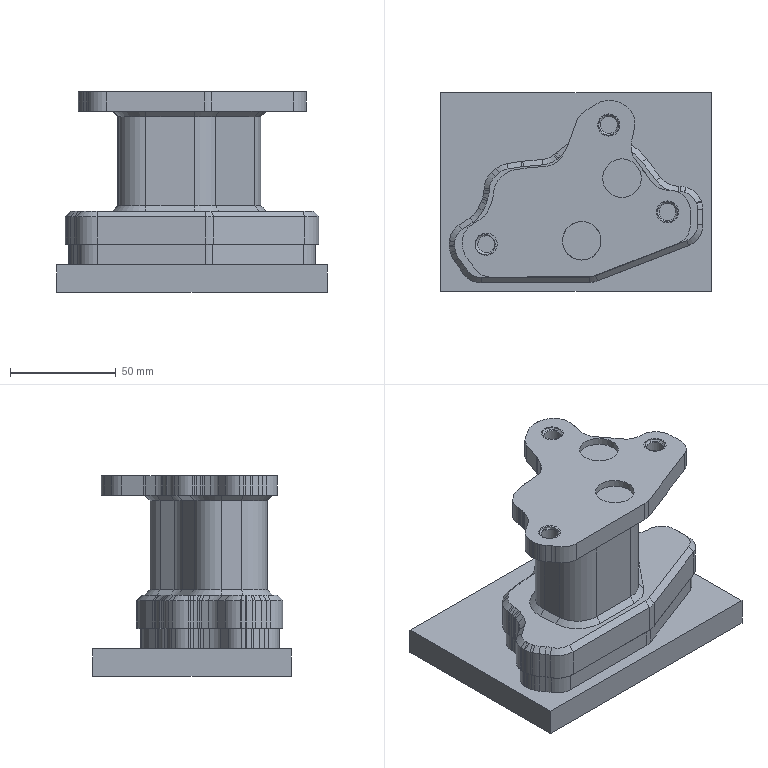Part | 3 solids | 552 faces | box 128.162 x 94.109 x 95 mm | volume 735256 mm3 | plane 266 | cylinder 159 | cone 123 | spline 4 | commonest cylinder face diameters 19.05 x66 21.188 x42 25.4 x14 17.68 x13 24.696 x8 9.525 x6